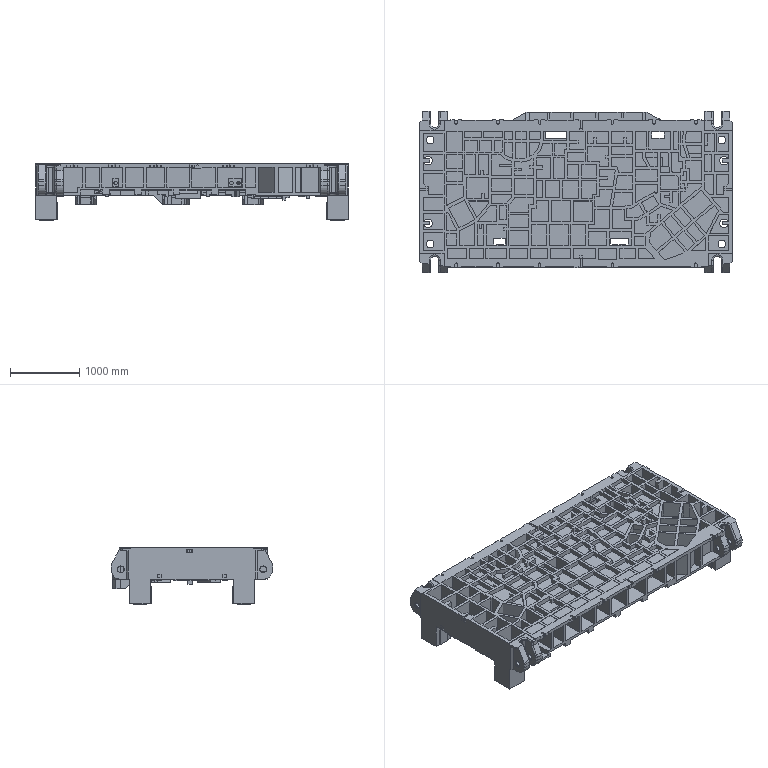Part | NX | features solid 2 | 1 solid | 2950 faces | box 4520 x 2330 x 810 mm | volume 1539345664 mm3 | plane 2453 | cylinder 260 | spline 211 | torus 24 | sphere 2 | commonest cylinder face diameters 100 x55 40 x42 25 x21 96 x16 30 x13 120 x12